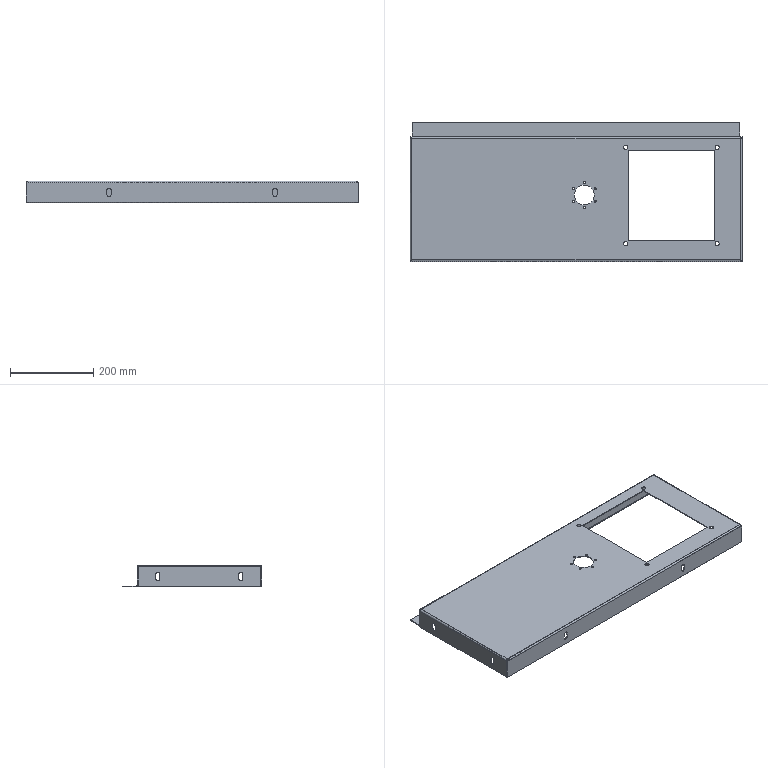Part | STEP file | SYL_0392D6J1SYL0380DJ1006_2_11X | 1 solid | 112 faces | box 800 x 335 x 53 mm | volume 648025 mm3 | plane 52 | cylinder 52 | spline 8 | commonest cylinder face diameters 10 x28 5 x12 4 x5 8 x5 48 x2